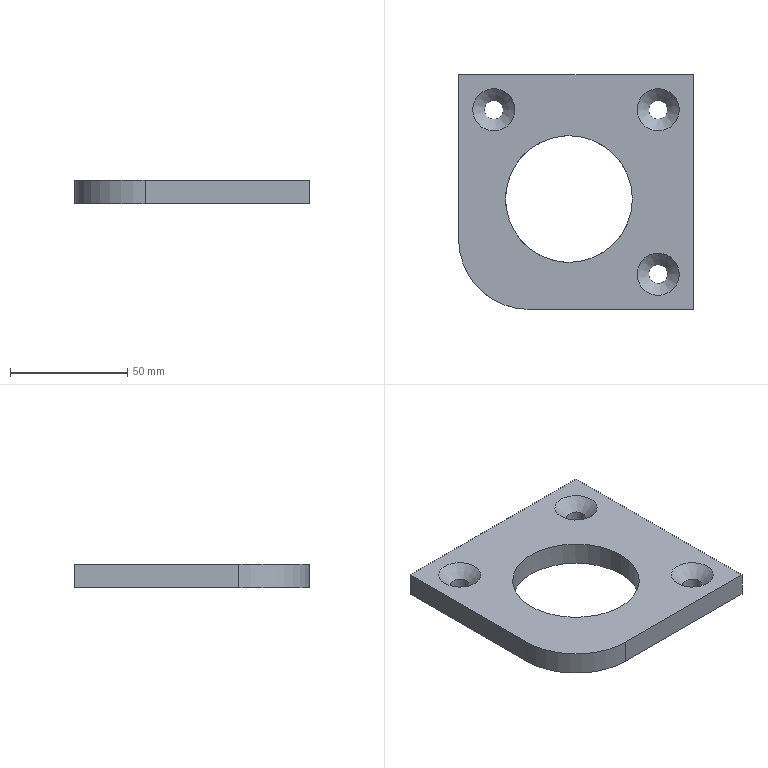Part | STEP file | solid 128 | 1 solid | 14 faces | box 100 x 100 x 10 mm | volume 72323 mm3 | plane 6 | cylinder 5 | cone 3 | commonest cylinder face diameters 8 x3 54 x1 60 x1